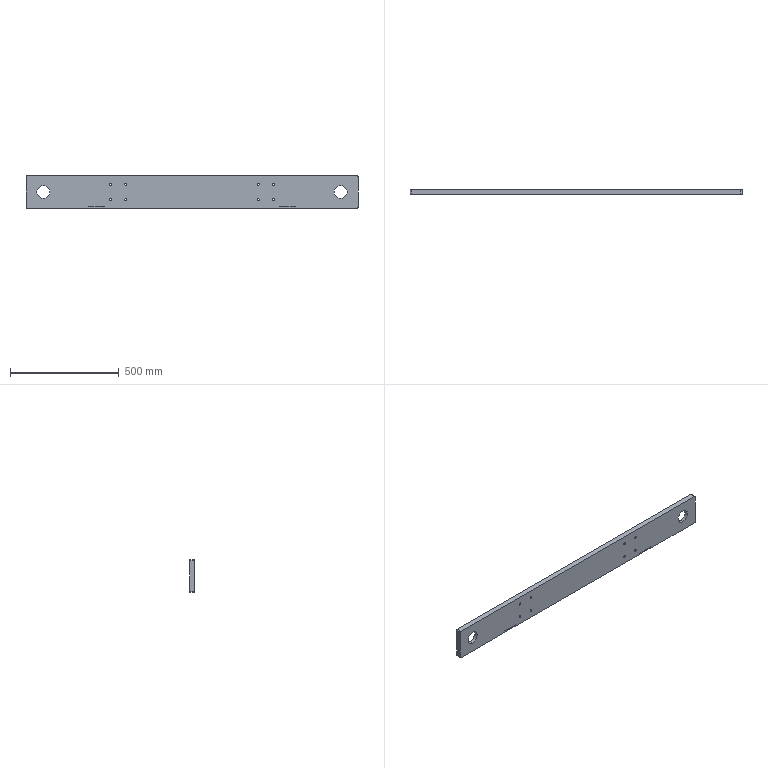Part | SolidWorks | features BaseBody 1 | 1 solid | 52 faces | box 1530 x 23 x 150 mm | volume 5107229 mm3 | cylinder 32 | plane 12 | cone 8 | commonest cylinder face diameters 10.2 x16 10 x8 60 x4 80 x4